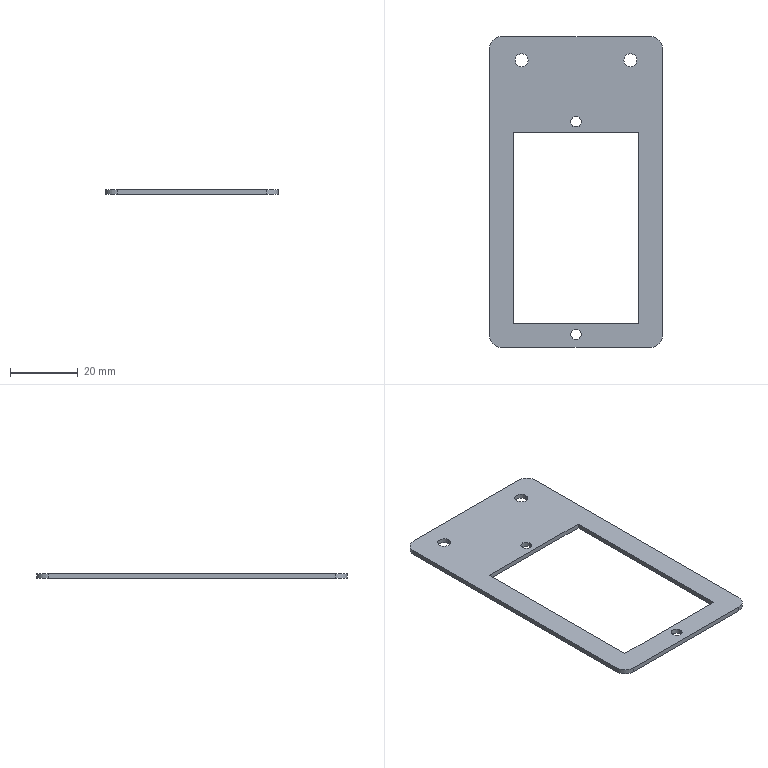Part | SolidWorks | features SplitBody 1 | 1 solid | 22 faces | box 51.1 x 92.05 x 1.4 mm | volume 3571 mm3 | cylinder 12 | plane 10 | commonest cylinder face diameters 3.15 x4 3.85 x4 7 x4
STEP:
#1=CARTESIAN_POINT('',(148.95,235.859,-257.316));
#2=VERTEX_POINT('',#1);
#3=CARTESIAN_POINT('',(152.8,235.859,-257.316));
#4=VERTEX_POINT('',#3);
#5=CARTESIAN_POINT('',(150.875,235.859,-257.316));
#6=DIRECTION('',(0.,0.,1.));
#7=DIRECTION('',(-1.,0.,0.));
#8=AXIS2_PLACEMENT_3D('',#5,#6,#7);
#9=CIRCLE('',#8,1.925);
#10=EDGE_CURVE('',#2,#4,#9,.T.);
#11=ORIENTED_EDGE('',*,*,#10,.F.);
#12=CARTESIAN_POINT('',(148.95,235.859,-255.916));
#13=VERTEX_POINT('',#12);
#14=CARTESIAN_POINT('',(148.95,235.859,-257.316));
#15=DIRECTION('',(0.,0.,1.));
#16=VECTOR('',#15,1000.);
#17=LINE('',#14,#16);
#18=EDGE_CURVE('',#2,#13,#17,.T.);
#19=ORIENTED_EDGE('',*,*,#18,.T.);
#20=CARTESIAN_POINT('',(152.8,235.859,-255.916));
#21=VERTEX_POINT('',#20);
#22=CARTESIAN_POINT('',(150.875,235.859,-255.916));
#23=DIRECTION('',(0.,0.,1.));
#24=DIRECTION('',(-1.,0.,0.));
#25=AXIS2_PLACEMENT_3D('',#22,#23,#24);
#26=CIRCLE('',#25,1.925);
#27=EDGE_CURVE('',#13,#21,#26,.T.);
#28=ORIENTED_EDGE('',*,*,#27,.T.);
#29=CARTESIAN_POINT('',(152.8,235.859,-257.316));
#30=DIRECTION('',(0.,0.,1.));
#31=VECTOR('',#30,1000.);
#32=LINE('',#29,#31);
#33=EDGE_CURVE('',#4,#21,#32,.T.);
#34=ORIENTED_EDGE('',*,*,#33,.F.);
#35=EDGE_LOOP('',(#11,#19,#28,#34));
#36=FACE_OUTER_BOUND('',#35,.T.);
#37=CARTESIAN_POINT('',(150.875,235.859,-257.316));
#38=DIRECTION('',(0.,0.,1.));
#39=DIRECTION('',(1.,0.,0.));
#40=AXIS2_PLACEMENT_3D('',#37,#38,#39);
#41=CYLINDRICAL_SURFACE('',#40,1.925);
#42=ADVANCED_FACE('',(#36),#41,.F.);
#43=CARTESIAN_POINT('',(116.75,235.859,-257.316));
#44=VERTEX_POINT('',#43);
#45=CARTESIAN_POINT('',(120.6,235.859,-257.316));
#46=VERTEX_POINT('',#45);
#47=CARTESIAN_POINT('',(118.675,235.859,-257.316));
#48=DIRECTION('',(0.,0.,1.));
#49=DIRECTION('',(1.,0.,0.));
#50=AXIS2_PLACEMENT_3D('',#47,#48,#49);
#51=CIRCLE('',#50,1.925);
#52=EDGE_CURVE('',#44,#46,#51,.T.);
#53=ORIENTED_EDGE('',*,*,#52,.F.);
#54=CARTESIAN_POINT('',(116.75,235.859,-255.916));
#55=VERTEX_POINT('',#54);
#56=CARTESIAN_POINT('',(116.75,235.859,-257.316));
#57=DIRECTION('',(0.,0.,1.));
#58=VECTOR('',#57,1000.);
#59=LINE('',#56,#58);
#60=EDGE_CURVE('',#44,#55,#59,.T.);
#61=ORIENTED_EDGE('',*,*,#60,.T.);
#62=CARTESIAN_POINT('',(120.6,235.859,-255.916));
#63=VERTEX_POINT('',#62);
#64=CARTESIAN_POINT('',(118.675,235.859,-255.916));
#65=DIRECTION('',(0.,0.,1.));
#66=DIRECTION('',(1.,0.,0.));
#67=AXIS2_PLACEMENT_3D('',#64,#65,#66);
#68=CIRCLE('',#67,1.925);
#69=EDGE_CURVE('',#55,#63,#68,.T.);
#70=ORIENTED_EDGE('',*,*,#69,.T.);
#71=CARTESIAN_POINT('',(120.6,235.859,-257.316));
#72=DIRECTION('',(0.,0.,1.));
#73=VECTOR('',#72,1000.);
#74=LINE('',#71,#73);
#75=EDGE_CURVE('',#46,#63,#74,.T.);
#76=ORIENTED_EDGE('',*,*,#75,.F.);
#77=EDGE_LOOP('',(#53,#61,#70,#76));
#78=FACE_OUTER_BOUND('',#77,.T.);
#79=CARTESIAN_POINT('',(118.675,235.859,-257.316));
#80=DIRECTION('',(0.,0.,1.));
#81=DIRECTION('',(1.,0.,0.));
#82=AXIS2_PLACEMENT_3D('',#79,#80,#81);
#83=CYLINDRICAL_SURFACE('',#82,1.925);
#84=ADVANCED_FACE('',(#78),#83,.F.);
#85=CARTESIAN_POINT('',(133.2,154.659,-257.316));
#86=VERTEX_POINT('',#85);
#87=CARTESIAN_POINT('',(136.35,154.659,-257.316));
#88=VERTEX_POINT('',#87);
#89=CARTESIAN_POINT('',(134.775,154.659,-257.316));
#90=DIRECTION('',(0.,0.,1.));
#91=DIRECTION('',(1.,0.,0.));
#92=AXIS2_PLACEMENT_3D('',#89,#90,#91);
#93=CIRCLE('',#92,1.575);
#94=EDGE_CURVE('',#86,#88,#93,.T.);
#95=ORIENTED_EDGE('',*,*,#94,.F.);
#96=CARTESIAN_POINT('',(133.2,154.659,-255.916));
#97=VERTEX_POINT('',#96);
#98=CARTESIAN_POINT('',(133.2,154.659,-257.316));
#99=DIRECTION('',(0.,0.,1.));
#100=VECTOR('',#99,1000.);
#101=LINE('',#98,#100);
#102=EDGE_CURVE('',#86,#97,#101,.T.);
#103=ORIENTED_EDGE('',*,*,#102,.T.);
#104=CARTESIAN_POINT('',(136.35,154.659,-255.916));
#105=VERTEX_POINT('',#104);
#106=CARTESIAN_POINT('',(134.775,154.659,-255.916));
#107=DIRECTION('',(0.,0.,1.));
#108=DIRECTION('',(1.,0.,0.));
#109=AXIS2_PLACEMENT_3D('',#106,#107,#108);
#110=CIRCLE('',#109,1.575);
#111=EDGE_CURVE('',#97,#105,#110,.T.);
#112=ORIENTED_EDGE('',*,*,#111,.T.);
#113=CARTESIAN_POINT('',(136.35,154.659,-257.316));
#114=DIRECTION('',(0.,0.,1.));
#115=VECTOR('',#114,1000.);
#116=LINE('',#113,#115);
#117=EDGE_CURVE('',#88,#105,#116,.T.);
#118=ORIENTED_EDGE('',*,*,#117,.F.);
#119=EDGE_LOOP('',(#95,#103,#112,#118));
#120=FACE_OUTER_BOUND('',#119,.T.);
#121=CARTESIAN_POINT('',(134.775,154.659,-257.316));
#122=DIRECTION('',(0.,0.,1.));
#123=DIRECTION('',(1.,0.,0.));
#124=AXIS2_PLACEMENT_3D('',#121,#122,#123);
#125=CYLINDRICAL_SURFACE('',#124,1.575);
#126=ADVANCED_FACE('',(#120),#125,.F.);
#127=CARTESIAN_POINT('',(133.2,217.659,-257.316));
#128=VERTEX_POINT('',#127);
#129=CARTESIAN_POINT('',(136.35,217.659,-257.316));
#130=VERTEX_POINT('',#129);
#131=CARTESIAN_POINT('',(134.775,217.659,-257.316));
#132=DIRECTION('',(0.,0.,1.));
#133=DIRECTION('',(1.,0.,0.));
#134=AXIS2_PLACEMENT_3D('',#131,#132,#133);
#135=CIRCLE('',#134,1.575);
#136=EDGE_CURVE('',#128,#130,#135,.T.);
#137=ORIENTED_EDGE('',*,*,#136,.F.);
#138=CARTESIAN_POINT('',(133.2,217.659,-255.916));
#139=VERTEX_POINT('',#138);
#140=CARTESIAN_POINT('',(133.2,217.659,-257.316));
#141=DIRECTION('',(0.,0.,1.));
#142=VECTOR('',#141,1000.);
#143=LINE('',#140,#142);
#144=EDGE_CURVE('',#128,#139,#143,.T.);
#145=ORIENTED_EDGE('',*,*,#144,.T.);
#146=CARTESIAN_POINT('',(136.35,217.659,-255.916));
#147=VERTEX_POINT('',#146);
#148=CARTESIAN_POINT('',(134.775,217.659,-255.916));
#149=DIRECTION('',(0.,0.,1.));
#150=DIRECTION('',(1.,0.,0.));
#151=AXIS2_PLACEMENT_3D('',#148,#149,#150);
#152=CIRCLE('',#151,1.575);
#153=EDGE_CURVE('',#139,#147,#152,.T.);
#154=ORIENTED_EDGE('',*,*,#153,.T.);
#155=CARTESIAN_POINT('',(136.35,217.659,-257.316));
#156=DIRECTION('',(0.,0.,1.));
#157=VECTOR('',#156,1000.);
#158=LINE('',#155,#157);
#159=EDGE_CURVE('',#130,#147,#158,.T.);
#160=ORIENTED_EDGE('',*,*,#159,.F.);
#161=EDGE_LOOP('',(#137,#145,#154,#160));
#162=FACE_OUTER_BOUND('',#161,.T.);
#163=CARTESIAN_POINT('',(134.775,217.659,-257.316));
#164=DIRECTION('',(0.,0.,1.));
#165=DIRECTION('',(1.,0.,0.));
#166=AXIS2_PLACEMENT_3D('',#163,#164,#165);
#167=CYLINDRICAL_SURFACE('',#166,1.575);
#168=ADVANCED_FACE('',(#162),#167,.F.);
#169=CARTESIAN_POINT('',(112.725,150.809,-257.316));
#170=VERTEX_POINT('',#169);
#171=CARTESIAN_POINT('',(156.825,150.809,-257.316));
#172=VERTEX_POINT('',#171);
#173=CARTESIAN_POINT('',(160.325,150.809,-257.316));
#174=DIRECTION('',(1.,0.,0.));
#175=VECTOR('',#174,1000.);
#176=LINE('',#173,#175);
#177=EDGE_CURVE('',#170,#172,#176,.T.);
#178=ORIENTED_EDGE('',*,*,#177,.F.);
#179=CARTESIAN_POINT('',(109.225,154.309,-257.316));
#180=VERTEX_POINT('',#179);
#181=CARTESIAN_POINT('',(112.725,154.309,-257.316));
#182=DIRECTION('',(0.,0.,-1.));
#183=DIRECTION('',(-1.,0.,0.));
#184=AXIS2_PLACEMENT_3D('',#181,#182,#183);
#185=CIRCLE('',#184,3.5);
#186=EDGE_CURVE('',#170,#180,#185,.T.);
#187=ORIENTED_EDGE('',*,*,#186,.T.);
#188=CARTESIAN_POINT('',(109.225,239.359,-257.316));
#189=VERTEX_POINT('',#188);
#190=CARTESIAN_POINT('',(109.225,227.459,-257.316));
#191=DIRECTION('',(0.,1.,0.));
#192=VECTOR('',#191,1000.);
#193=LINE('',#190,#192);
#194=EDGE_CURVE('',#180,#189,#193,.T.);
#195=ORIENTED_EDGE('',*,*,#194,.T.);
#196=CARTESIAN_POINT('',(112.725,242.859,-257.316));
#197=VERTEX_POINT('',#196);
#198=CARTESIAN_POINT('',(112.725,239.359,-257.316));
#199=DIRECTION('',(0.,0.,-1.));
#200=DIRECTION('',(-1.,0.,0.));
#201=AXIS2_PLACEMENT_3D('',#198,#199,#200);
#202=CIRCLE('',#201,3.5);
#203=EDGE_CURVE('',#189,#197,#202,.T.);
#204=ORIENTED_EDGE('',*,*,#203,.T.);
#205=CARTESIAN_POINT('',(156.825,242.859,-257.316));
#206=VERTEX_POINT('',#205);
#207=CARTESIAN_POINT('',(160.325,242.859,-257.316));
#208=DIRECTION('',(1.,0.,0.));
#209=VECTOR('',#208,1000.);
#210=LINE('',#207,#209);
#211=EDGE_CURVE('',#197,#206,#210,.T.);
#212=ORIENTED_EDGE('',*,*,#211,.T.);
#213=CARTESIAN_POINT('',(160.325,239.359,-257.316));
#214=VERTEX_POINT('',#213);
#215=CARTESIAN_POINT('',(156.825,239.359,-257.316));
#216=DIRECTION('',(0.,0.,-1.));
#217=DIRECTION('',(-1.,0.,0.));
#218=AXIS2_PLACEMENT_3D('',#215,#216,#217);
#219=CIRCLE('',#218,3.5);
#220=EDGE_CURVE('',#206,#214,#219,.T.);
#221=ORIENTED_EDGE('',*,*,#220,.T.);
#222=CARTESIAN_POINT('',(160.325,154.309,-257.316));
#223=VERTEX_POINT('',#222);
#224=CARTESIAN_POINT('',(160.325,227.459,-257.316));
#225=DIRECTION('',(0.,-1.,0.));
#226=VECTOR('',#225,1000.);
#227=LINE('',#224,#226);
#228=EDGE_CURVE('',#214,#223,#227,.T.);
#229=ORIENTED_EDGE('',*,*,#228,.T.);
#230=CARTESIAN_POINT('',(156.825,154.309,-257.316));
#231=DIRECTION('',(0.,0.,-1.));
#232=DIRECTION('',(-1.,0.,0.));
#233=AXIS2_PLACEMENT_3D('',#230,#231,#232);
#234=CIRCLE('',#233,3.5);
#235=EDGE_CURVE('',#223,#172,#234,.T.);
#236=ORIENTED_EDGE('',*,*,#235,.T.);
#237=EDGE_LOOP('',(#178,#187,#195,#204,#212,#221,#229,#236));
#238=FACE_OUTER_BOUND('',#237,.T.);
#239=CARTESIAN_POINT('',(150.875,235.859,-257.316));
#240=DIRECTION('',(0.,0.,1.));
#241=DIRECTION('',(-1.,0.,0.));
#242=AXIS2_PLACEMENT_3D('',#239,#240,#241);
#243=CIRCLE('',#242,1.925);
#244=EDGE_CURVE('',#4,#2,#243,.T.);
#245=ORIENTED_EDGE('',*,*,#244,.T.);
#246=ORIENTED_EDGE('',*,*,#10,.T.);
#247=EDGE_LOOP('',(#245,#246));
#248=FACE_BOUND('',#247,.T.);
#249=CARTESIAN_POINT('',(118.675,235.859,-257.316));
#250=DIRECTION('',(0.,0.,1.));
#251=DIRECTION('',(1.,0.,0.));
#252=AXIS2_PLACEMENT_3D('',#249,#250,#251);
#253=CIRCLE('',#252,1.925);
#254=EDGE_CURVE('',#46,#44,#253,.T.);
#255=ORIENTED_EDGE('',*,*,#254,.T.);
#256=ORIENTED_EDGE('',*,*,#52,.T.);
#257=EDGE_LOOP('',(#255,#256));
#258=FACE_BOUND('',#257,.T.);
#259=CARTESIAN_POINT('',(134.775,154.659,-257.316));
#260=DIRECTION('',(0.,0.,1.));
#261=DIRECTION('',(1.,0.,0.));
#262=AXIS2_PLACEMENT_3D('',#259,#260,#261);
#263=CIRCLE('',#262,1.575);
#264=EDGE_CURVE('',#88,#86,#263,.T.);
#265=ORIENTED_EDGE('',*,*,#264,.T.);
#266=ORIENTED_EDGE('',*,*,#94,.T.);
#267=EDGE_LOOP('',(#265,#266));
#268=FACE_BOUND('',#267,.T.);
#269=CARTESIAN_POINT('',(134.775,217.659,-257.316));
#270=DIRECTION('',(0.,0.,1.));
#271=DIRECTION('',(1.,0.,0.));
#272=AXIS2_PLACEMENT_3D('',#269,#270,#271);
#273=CIRCLE('',#272,1.575);
#274=EDGE_CURVE('',#130,#128,#273,.T.);
#275=ORIENTED_EDGE('',*,*,#274,.T.);
#276=ORIENTED_EDGE('',*,*,#136,.T.);
#277=EDGE_LOOP('',(#275,#276));
#278=FACE_BOUND('',#277,.T.);
#279=CARTESIAN_POINT('',(153.325,214.509,-257.316));
#280=VERTEX_POINT('',#279);
#281=CARTESIAN_POINT('',(153.325,157.809,-257.316));
#282=VERTEX_POINT('',#281);
#283=CARTESIAN_POINT('',(153.325,220.459,-257.316));
#284=DIRECTION('',(0.,-1.,0.));
#285=VECTOR('',#284,1000.);
#286=LINE('',#283,#285);
#287=EDGE_CURVE('',#280,#282,#286,.T.);
#288=ORIENTED_EDGE('',*,*,#287,.F.);
#289=CARTESIAN_POINT('',(116.225,214.509,-257.316));
#290=VERTEX_POINT('',#289);
#291=CARTESIAN_POINT('',(153.325,214.509,-257.316));
#292=DIRECTION('',(-1.,0.,0.));
#293=VECTOR('',#292,1000.);
#294=LINE('',#291,#293);
#295=EDGE_CURVE('',#280,#290,#294,.T.);
#296=ORIENTED_EDGE('',*,*,#295,.T.);
#297=CARTESIAN_POINT('',(116.225,157.809,-257.316));
#298=VERTEX_POINT('',#297);
#299=CARTESIAN_POINT('',(116.225,220.459,-257.316));
#300=DIRECTION('',(0.,1.,0.));
#301=VECTOR('',#300,1000.);
#302=LINE('',#299,#301);
#303=EDGE_CURVE('',#298,#290,#302,.T.);
#304=ORIENTED_EDGE('',*,*,#303,.F.);
#305=CARTESIAN_POINT('',(153.325,157.809,-257.316));
#306=DIRECTION('',(1.,0.,0.));
#307=VECTOR('',#306,1000.);
#308=LINE('',#305,#307);
#309=EDGE_CURVE('',#298,#282,#308,.T.);
#310=ORIENTED_EDGE('',*,*,#309,.T.);
#311=EDGE_LOOP('',(#288,#296,#304,#310));
#312=FACE_BOUND('',#311,.T.);
#313=CARTESIAN_POINT('',(160.325,144.859,-257.316));
#314=DIRECTION('',(0.,0.,-1.));
#315=DIRECTION('',(-1.,0.,0.));
#316=AXIS2_PLACEMENT_3D('',#313,#314,#315);
#317=PLANE('',#316);
#318=ADVANCED_FACE('',(#238,#248,#258,#268,#278,#312),#317,.T.);
#319=CARTESIAN_POINT('',(150.875,235.859,-255.916));
#320=DIRECTION('',(0.,0.,1.));
#321=DIRECTION('',(-1.,0.,0.));
#322=AXIS2_PLACEMENT_3D('',#319,#320,#321);
#323=CIRCLE('',#322,1.925);
#324=EDGE_CURVE('',#21,#13,#323,.T.);
#325=ORIENTED_EDGE('',*,*,#324,.F.);
#326=ORIENTED_EDGE('',*,*,#27,.F.);
#327=EDGE_LOOP('',(#325,#326));
#328=FACE_BOUND('',#327,.T.);
#329=CARTESIAN_POINT('',(118.675,235.859,-255.916));
#330=DIRECTION('',(0.,0.,1.));
#331=DIRECTION('',(1.,0.,0.));
#332=AXIS2_PLACEMENT_3D('',#329,#330,#331);
#333=CIRCLE('',#332,1.925);
#334=EDGE_CURVE('',#63,#55,#333,.T.);
#335=ORIENTED_EDGE('',*,*,#334,.F.);
#336=ORIENTED_EDGE('',*,*,#69,.F.);
#337=EDGE_LOOP('',(#335,#336));
#338=FACE_BOUND('',#337,.T.);
#339=CARTESIAN_POINT('',(134.775,154.659,-255.916));
#340=DIRECTION('',(0.,0.,1.));
#341=DIRECTION('',(1.,0.,0.));
#342=AXIS2_PLACEMENT_3D('',#339,#340,#341);
#343=CIRCLE('',#342,1.575);
#344=EDGE_CURVE('',#105,#97,#343,.T.);
#345=ORIENTED_EDGE('',*,*,#344,.F.);
#346=ORIENTED_EDGE('',*,*,#111,.F.);
#347=EDGE_LOOP('',(#345,#346));
#348=FACE_BOUND('',#347,.T.);
#349=CARTESIAN_POINT('',(134.775,217.659,-255.916));
#350=DIRECTION('',(0.,0.,1.));
#351=DIRECTION('',(1.,0.,0.));
#352=AXIS2_PLACEMENT_3D('',#349,#350,#351);
#353=CIRCLE('',#352,1.575);
#354=EDGE_CURVE('',#147,#139,#353,.T.);
#355=ORIENTED_EDGE('',*,*,#354,.F.);
#356=ORIENTED_EDGE('',*,*,#153,.F.);
#357=EDGE_LOOP('',(#355,#356));
#358=FACE_BOUND('',#357,.T.);
#359=CARTESIAN_POINT('',(116.225,214.509,-255.916));
#360=VERTEX_POINT('',#359);
#361=CARTESIAN_POINT('',(153.325,214.509,-255.916));
#362=VERTEX_POINT('',#361);
#363=CARTESIAN_POINT('',(153.325,214.509,-255.916));
#364=DIRECTION('',(1.,0.,0.));
#365=VECTOR('',#364,1000.);
#366=LINE('',#363,#365);
#367=EDGE_CURVE('',#360,#362,#366,.T.);
#368=ORIENTED_EDGE('',*,*,#367,.T.);
#369=CARTESIAN_POINT('',(153.325,157.809,-255.916));
#370=VERTEX_POINT('',#369);
#371=CARTESIAN_POINT('',(153.325,220.459,-255.916));
#372=DIRECTION('',(0.,-1.,0.));
#373=VECTOR('',#372,1000.);
#374=LINE('',#371,#373);
#375=EDGE_CURVE('',#362,#370,#374,.T.);
#376=ORIENTED_EDGE('',*,*,#375,.T.);
#377=CARTESIAN_POINT('',(116.225,157.809,-255.916));
#378=VERTEX_POINT('',#377);
#379=CARTESIAN_POINT('',(153.325,157.809,-255.916));
#380=DIRECTION('',(-1.,0.,0.));
#381=VECTOR('',#380,1000.);
#382=LINE('',#379,#381);
#383=EDGE_CURVE('',#370,#378,#382,.T.);
#384=ORIENTED_EDGE('',*,*,#383,.T.);
#385=CARTESIAN_POINT('',(116.225,220.459,-255.916));
#386=DIRECTION('',(0.,1.,0.));
#387=VECTOR('',#386,1000.);
#388=LINE('',#385,#387);
#389=EDGE_CURVE('',#378,#360,#388,.T.);
#390=ORIENTED_EDGE('',*,*,#389,.T.);
#391=EDGE_LOOP('',(#368,#376,#384,#390));
#392=FACE_BOUND('',#391,.T.);
#393=CARTESIAN_POINT('',(109.225,154.309,-255.916));
#394=VERTEX_POINT('',#393);
#395=CARTESIAN_POINT('',(109.225,239.359,-255.916));
#396=VERTEX_POINT('',#395);
#397=CARTESIAN_POINT('',(109.225,227.459,-255.916));
#398=DIRECTION('',(0.,1.,0.));
#399=VECTOR('',#398,1000.);
#400=LINE('',#397,#399);
#401=EDGE_CURVE('',#394,#396,#400,.T.);
#402=ORIENTED_EDGE('',*,*,#401,.F.);
#403=CARTESIAN_POINT('',(112.725,150.809,-255.916));
#404=VERTEX_POINT('',#403);
#405=CARTESIAN_POINT('',(112.725,154.309,-255.916));
#406=DIRECTION('',(0.,0.,1.));
#407=DIRECTION('',(-1.,0.,0.));
#408=AXIS2_PLACEMENT_3D('',#405,#406,#407);
#409=CIRCLE('',#408,3.5);
#410=EDGE_CURVE('',#394,#404,#409,.T.);
#411=ORIENTED_EDGE('',*,*,#410,.T.);
#412=CARTESIAN_POINT('',(156.825,150.809,-255.916));
#413=VERTEX_POINT('',#412);
#414=CARTESIAN_POINT('',(160.325,150.809,-255.916));
#415=DIRECTION('',(1.,0.,0.));
#416=VECTOR('',#415,1000.);
#417=LINE('',#414,#416);
#418=EDGE_CURVE('',#404,#413,#417,.T.);
#419=ORIENTED_EDGE('',*,*,#418,.T.);
#420=CARTESIAN_POINT('',(160.325,154.309,-255.916));
#421=VERTEX_POINT('',#420);
#422=CARTESIAN_POINT('',(156.825,154.309,-255.916));
#423=DIRECTION('',(0.,0.,1.));
#424=DIRECTION('',(-1.,0.,0.));
#425=AXIS2_PLACEMENT_3D('',#422,#423,#424);
#426=CIRCLE('',#425,3.5);
#427=EDGE_CURVE('',#413,#421,#426,.T.);
#428=ORIENTED_EDGE('',*,*,#427,.T.);
#429=CARTESIAN_POINT('',(160.325,239.359,-255.916));
#430=VERTEX_POINT('',#429);
#431=CARTESIAN_POINT('',(160.325,227.459,-255.916));
#432=DIRECTION('',(0.,-1.,0.));
#433=VECTOR('',#432,1000.);
#434=LINE('',#431,#433);
#435=EDGE_CURVE('',#430,#421,#434,.T.);
#436=ORIENTED_EDGE('',*,*,#435,.F.);
#437=CARTESIAN_POINT('',(156.825,242.859,-255.916));
#438=VERTEX_POINT('',#437);
#439=CARTESIAN_POINT('',(156.825,239.359,-255.916));
#440=DIRECTION('',(0.,0.,1.));
#441=DIRECTION('',(-1.,0.,0.));
#442=AXIS2_PLACEMENT_3D('',#439,#440,#441);
#443=CIRCLE('',#442,3.5);
#444=EDGE_CURVE('',#430,#438,#443,.T.);
#445=ORIENTED_EDGE('',*,*,#444,.T.);
#446=CARTESIAN_POINT('',(112.725,242.859,-255.916));
#447=VERTEX_POINT('',#446);
#448=CARTESIAN_POINT('',(160.325,242.859,-255.916));
#449=DIRECTION('',(-1.,0.,0.));
#450=VECTOR('',#449,1000.);
#451=LINE('',#448,#450);
#452=EDGE_CURVE('',#438,#447,#451,.T.);
#453=ORIENTED_EDGE('',*,*,#452,.T.);
#454=CARTESIAN_POINT('',(112.725,239.359,-255.916));
#455=DIRECTION('',(0.,0.,1.));
#456=DIRECTION('',(-1.,0.,0.));
#457=AXIS2_PLACEMENT_3D('',#454,#455,#456);
#458=CIRCLE('',#457,3.5);
#459=EDGE_CURVE('',#447,#396,#458,.T.);
#460=ORIENTED_EDGE('',*,*,#459,.T.);
#461=EDGE_LOOP('',(#402,#411,#419,#428,#436,#445,#453,#460));
#462=FACE_OUTER_BOUND('',#461,.T.);
#463=CARTESIAN_POINT('',(160.325,144.859,-255.916));
#464=DIRECTION('',(0.,0.,-1.));
#465=DIRECTION('',(-1.,0.,0.));
#466=AXIS2_PLACEMENT_3D('',#463,#464,#465);
#467=PLANE('',#466);
#468=ADVANCED_FACE('',(#328,#338,#348,#358,#392,#462),#467,.F.);
#469=ORIENTED_EDGE('',*,*,#435,.T.);
#470=CARTESIAN_POINT('',(160.325,154.309,-257.316));
#471=DIRECTION('',(0.,0.,-1.));
#472=VECTOR('',#471,1000.);
#473=LINE('',#470,#472);
#474=EDGE_CURVE('',#421,#223,#473,.T.);
#475=ORIENTED_EDGE('',*,*,#474,.T.);
#476=ORIENTED_EDGE('',*,*,#228,.F.);
#477=CARTESIAN_POINT('',(160.325,239.359,-255.916));
#478=DIRECTION('',(0.,0.,1.));
#479=VECTOR('',#478,1000.);
#480=LINE('',#477,#479);
#481=EDGE_CURVE('',#214,#430,#480,.T.);
#482=ORIENTED_EDGE('',*,*,#481,.T.);
#483=EDGE_LOOP('',(#469,#475,#476,#482));
#484=FACE_OUTER_BOUND('',#483,.T.);
#485=CARTESIAN_POINT('',(160.325,227.459,-257.316));
#486=DIRECTION('',(-1.,0.,0.));
#487=DIRECTION('',(0.,0.,1.));
#488=AXIS2_PLACEMENT_3D('',#485,#486,#487);
#489=PLANE('',#488);
#490=ADVANCED_FACE('',(#484),#489,.F.);
#491=ORIENTED_EDGE('',*,*,#194,.F.);
#492=CARTESIAN_POINT('',(109.225,154.309,-257.316));
#493=DIRECTION('',(0.,0.,1.));
#494=VECTOR('',#493,1000.);
#495=LINE('',#492,#494);
#496=EDGE_CURVE('',#180,#394,#495,.T.);
#497=ORIENTED_EDGE('',*,*,#496,.T.);
#498=ORIENTED_EDGE('',*,*,#401,.T.);
#499=CARTESIAN_POINT('',(109.225,239.359,-257.316));
#500=DIRECTION('',(0.,0.,-1.));
#501=VECTOR('',#500,1000.);
#502=LINE('',#499,#501);
#503=EDGE_CURVE('',#396,#189,#502,.T.);
#504=ORIENTED_EDGE('',*,*,#503,.T.);
#505=EDGE_LOOP('',(#491,#497,#498,#504));
#506=FACE_OUTER_BOUND('',#505,.T.);
#507=CARTESIAN_POINT('',(109.225,227.459,-257.316));
#508=DIRECTION('',(1.,0.,0.));
#509=DIRECTION('',(0.,0.,-1.));
#510=AXIS2_PLACEMENT_3D('',#507,#508,#509);
#511=PLANE('',#510);
#512=ADVANCED_FACE('',(#506),#511,.F.);
#513=CARTESIAN_POINT('',(153.325,214.509,-218.342));
#514=DIRECTION('',(0.,0.,-1.));
#515=VECTOR('',#514,1000.);
#516=LINE('',#513,#515);
#517=EDGE_CURVE('',#362,#280,#516,.T.);
#518=ORIENTED_EDGE('',*,*,#517,.T.);
#519=ORIENTED_EDGE('',*,*,#287,.T.);
#520=CARTESIAN_POINT('',(153.325,157.809,-218.342));
#521=DIRECTION('',(0.,0.,-1.));
#522=VECTOR('',#521,1000.);
#523=LINE('',#520,#522);
#524=EDGE_CURVE('',#370,#282,#523,.T.);
#525=ORIENTED_EDGE('',*,*,#524,.F.);
#526=ORIENTED_EDGE('',*,*,#375,.F.);
#527=EDGE_LOOP('',(#518,#519,#525,#526));
#528=FACE_OUTER_BOUND('',#527,.T.);
#529=CARTESIAN_POINT('',(153.325,220.459,-257.316));
#530=DIRECTION('',(-1.,0.,0.));
#531=DIRECTION('',(0.,1.,0.));
#532=AXIS2_PLACEMENT_3D('',#529,#530,#531);
#533=PLANE('',#532);
#534=ADVANCED_FACE('',(#528),#533,.T.);
#535=CARTESIAN_POINT('',(116.225,214.509,-218.342));
#536=DIRECTION('',(0.,0.,-1.));
#537=VECTOR('',#536,1000.);
#538=LINE('',#535,#537);
#539=EDGE_CURVE('',#360,#290,#538,.T.);
#540=ORIENTED_EDGE('',*,*,#539,.F.);
#541=ORIENTED_EDGE('',*,*,#389,.F.);
#542=CARTESIAN_POINT('',(116.225,157.809,-218.342));
#543=DIRECTION('',(0.,0.,-1.));
#544=VECTOR('',#543,1000.);
#545=LINE('',#542,#544);
#546=EDGE_CURVE('',#378,#298,#545,.T.);
#547=ORIENTED_EDGE('',*,*,#546,.T.);
#548=ORIENTED_EDGE('',*,*,#303,.T.);
#549=EDGE_LOOP('',(#540,#541,#547,#548));
#550=FACE_OUTER_BOUND('',#549,.T.);
#551=CARTESIAN_POINT('',(116.225,220.459,-257.316));
#552=DIRECTION('',(1.,0.,0.));
#553=DIRECTION('',(0.,0.,-1.));
#554=AXIS2_PLACEMENT_3D('',#551,#552,#553);
#555=PLANE('',#554);
#556=ADVANCED_FACE('',(#550),#555,.T.);
#557=ORIENTED_EDGE('',*,*,#383,.F.);
#558=ORIENTED_EDGE('',*,*,#524,.T.);
#559=ORIENTED_EDGE('',*,*,#309,.F.);
#560=ORIENTED_EDGE('',*,*,#546,.F.);
#561=EDGE_LOOP('',(#557,#558,#559,#560));
#562=FACE_OUTER_BOUND('',#561,.T.);
#563=CARTESIAN_POINT('',(153.325,157.809,-218.342));
#564=DIRECTION('',(0.,1.,0.));
#565=DIRECTION('',(0.,0.,-1.));
#566=AXIS2_PLACEMENT_3D('',#563,#564,#565);
#567=PLANE('',#566);
#568=ADVANCED_FACE('',(#562),#567,.T.);
#569=ORIENTED_EDGE('',*,*,#367,.F.);
#570=ORIENTED_EDGE('',*,*,#539,.T.);
#571=ORIENTED_EDGE('',*,*,#295,.F.);
#572=ORIENTED_EDGE('',*,*,#517,.F.);
#573=EDGE_LOOP('',(#569,#570,#571,#572));
#574=FACE_OUTER_BOUND('',#573,.T.);
#575=CARTESIAN_POINT('',(153.325,214.509,-218.342));
#576=DIRECTION('',(0.,-1.,0.));
#577=DIRECTION('',(-1.,0.,0.));
#578=AXIS2_PLACEMENT_3D('',#575,#576,#577);
#579=PLANE('',#578);
#580=ADVANCED_FACE('',(#574),#579,.T.);
#581=ORIENTED_EDGE('',*,*,#211,.F.);
#582=CARTESIAN_POINT('',(112.725,242.859,-255.916));
#583=DIRECTION('',(0.,0.,1.));
#584=VECTOR('',#583,1000.);
#585=LINE('',#582,#584);
#586=EDGE_CURVE('',#197,#447,#585,.T.);
#587=ORIENTED_EDGE('',*,*,#586,.T.);
#588=ORIENTED_EDGE('',*,*,#452,.F.);
#589=CARTESIAN_POINT('',(156.825,242.859,-257.316));
#590=DIRECTION('',(0.,0.,-1.));
#591=VECTOR('',#590,1000.);
#592=LINE('',#589,#591);
#593=EDGE_CURVE('',#438,#206,#592,.T.);
#594=ORIENTED_EDGE('',*,*,#593,.T.);
#595=EDGE_LOOP('',(#581,#587,#588,#594));
#596=FACE_OUTER_BOUND('',#595,.T.);
#597=CARTESIAN_POINT('',(160.325,242.859,-202.545));
#598=DIRECTION('',(0.,1.,0.));
#599=DIRECTION('',(0.,0.,-1.));
#600=AXIS2_PLACEMENT_3D('',#597,#598,#599);
#601=PLANE('',#600);
#602=ADVANCED_FACE('',(#596),#601,.T.);
#603=ORIENTED_EDGE('',*,*,#459,.F.);
#604=ORIENTED_EDGE('',*,*,#586,.F.);
#605=ORIENTED_EDGE('',*,*,#203,.F.);
#606=ORIENTED_EDGE('',*,*,#503,.F.);
#607=EDGE_LOOP('',(#603,#604,#605,#606));
#608=FACE_OUTER_BOUND('',#607,.T.);
#609=CARTESIAN_POINT('',(112.725,239.359,-257.316));
#610=DIRECTION('',(0.,0.,1.));
#611=DIRECTION('',(1.,0.,0.));
#612=AXIS2_PLACEMENT_3D('',#609,#610,#611);
#613=CYLINDRICAL_SURFACE('',#612,3.5);
#614=ADVANCED_FACE('',(#608),#613,.T.);
#615=ORIENTED_EDGE('',*,*,#444,.F.);
#616=ORIENTED_EDGE('',*,*,#481,.F.);
#617=ORIENTED_EDGE('',*,*,#220,.F.);
#618=ORIENTED_EDGE('',*,*,#593,.F.);
#619=EDGE_LOOP('',(#615,#616,#617,#618));
#620=FACE_OUTER_BOUND('',#619,.T.);
#621=CARTESIAN_POINT('',(156.825,239.359,-202.545));
#622=DIRECTION('',(0.,0.,1.));
#623=DIRECTION('',(1.,0.,0.));
#624=AXIS2_PLACEMENT_3D('',#621,#622,#623);
#625=CYLINDRICAL_SURFACE('',#624,3.5);
#626=ADVANCED_FACE('',(#620),#625,.T.);
#627=ORIENTED_EDGE('',*,*,#144,.F.);
#628=ORIENTED_EDGE('',*,*,#274,.F.);
#629=ORIENTED_EDGE('',*,*,#159,.T.);
#630=ORIENTED_EDGE('',*,*,#354,.T.);
#631=EDGE_LOOP('',(#627,#628,#629,#630));
#632=FACE_OUTER_BOUND('',#631,.T.);
#633=CARTESIAN_POINT('',(134.775,217.659,-257.316));
#634=DIRECTION('',(0.,0.,1.));
#635=DIRECTION('',(1.,0.,0.));
#636=AXIS2_PLACEMENT_3D('',#633,#634,#635);
#637=CYLINDRICAL_SURFACE('',#636,1.575);
#638=ADVANCED_FACE('',(#632),#637,.F.);
#639=ORIENTED_EDGE('',*,*,#102,.F.);
#640=ORIENTED_EDGE('',*,*,#264,.F.);
#641=ORIENTED_EDGE('',*,*,#117,.T.);
#642=ORIENTED_EDGE('',*,*,#344,.T.);
#643=EDGE_LOOP('',(#639,#640,#641,#642));
#644=FACE_OUTER_BOUND('',#643,.T.);
#645=CARTESIAN_POINT('',(134.775,154.659,-257.316));
#646=DIRECTION('',(0.,0.,1.));
#647=DIRECTION('',(1.,0.,0.));
#648=AXIS2_PLACEMENT_3D('',#645,#646,#647);
#649=CYLINDRICAL_SURFACE('',#648,1.575);
#650=ADVANCED_FACE('',(#644),#649,.F.);
#651=ORIENTED_EDGE('',*,*,#60,.F.);
#652=ORIENTED_EDGE('',*,*,#254,.F.);
#653=ORIENTED_EDGE('',*,*,#75,.T.);
#654=ORIENTED_EDGE('',*,*,#334,.T.);
#655=EDGE_LOOP('',(#651,#652,#653,#654));
#656=FACE_OUTER_BOUND('',#655,.T.);
#657=CARTESIAN_POINT('',(118.675,235.859,-257.316));
#658=DIRECTION('',(0.,0.,1.));
#659=DIRECTION('',(1.,0.,0.));
#660=AXIS2_PLACEMENT_3D('',#657,#658,#659);
#661=CYLINDRICAL_SURFACE('',#660,1.925);
#662=ADVANCED_FACE('',(#656),#661,.F.);
#663=ORIENTED_EDGE('',*,*,#18,.F.);
#664=ORIENTED_EDGE('',*,*,#244,.F.);
#665=ORIENTED_EDGE('',*,*,#33,.T.);
#666=ORIENTED_EDGE('',*,*,#324,.T.);
#667=EDGE_LOOP('',(#663,#664,#665,#666));
#668=FACE_OUTER_BOUND('',#667,.T.);
#669=CARTESIAN_POINT('',(150.875,235.859,-257.316));
#670=DIRECTION('',(0.,0.,1.));
#671=DIRECTION('',(1.,0.,0.));
#672=AXIS2_PLACEMENT_3D('',#669,#670,#671);
#673=CYLINDRICAL_SURFACE('',#672,1.925);
#674=ADVANCED_FACE('',(#668),#673,.F.);
#675=ORIENTED_EDGE('',*,*,#418,.F.);
#676=CARTESIAN_POINT('',(112.725,150.809,-250.316));
#677=DIRECTION('',(0.,0.,-1.));
#678=VECTOR('',#677,1000.);
#679=LINE('',#676,#678);
#680=EDGE_CURVE('',#404,#170,#679,.T.);
#681=ORIENTED_EDGE('',*,*,#680,.T.);
#682=ORIENTED_EDGE('',*,*,#177,.T.);
#683=CARTESIAN_POINT('',(156.825,150.809,-250.316));
#684=DIRECTION('',(0.,0.,1.));
#685=VECTOR('',#684,1000.);
#686=LINE('',#683,#685);
#687=EDGE_CURVE('',#172,#413,#686,.T.);
#688=ORIENTED_EDGE('',*,*,#687,.T.);
#689=EDGE_LOOP('',(#675,#681,#682,#688));
#690=FACE_OUTER_BOUND('',#689,.T.);
#691=CARTESIAN_POINT('',(160.325,150.809,-250.316));
#692=DIRECTION('',(0.,1.,0.));
#693=DIRECTION('',(1.,0.,0.));
#694=AXIS2_PLACEMENT_3D('',#691,#692,#693);
#695=PLANE('',#694);
#696=ADVANCED_FACE('',(#690),#695,.F.);
#697=ORIENTED_EDGE('',*,*,#186,.F.);
#698=ORIENTED_EDGE('',*,*,#680,.F.);
#699=ORIENTED_EDGE('',*,*,#410,.F.);
#700=ORIENTED_EDGE('',*,*,#496,.F.);
#701=EDGE_LOOP('',(#697,#698,#699,#700));
#702=FACE_OUTER_BOUND('',#701,.T.);
#703=CARTESIAN_POINT('',(112.725,154.309,-257.316));
#704=DIRECTION('',(0.,0.,1.));
#705=DIRECTION('',(1.,0.,0.));
#706=AXIS2_PLACEMENT_3D('',#703,#704,#705);
#707=CYLINDRICAL_SURFACE('',#706,3.5);
#708=ADVANCED_FACE('',(#702),#707,.T.);
#709=ORIENTED_EDGE('',*,*,#427,.F.);
#710=ORIENTED_EDGE('',*,*,#687,.F.);
#711=ORIENTED_EDGE('',*,*,#235,.F.);
#712=ORIENTED_EDGE('',*,*,#474,.F.);
#713=EDGE_LOOP('',(#709,#710,#711,#712));
#714=FACE_OUTER_BOUND('',#713,.T.);
#715=CARTESIAN_POINT('',(156.825,154.309,-257.316));
#716=DIRECTION('',(0.,0.,-1.));
#717=DIRECTION('',(-1.,0.,0.));
#718=AXIS2_PLACEMENT_3D('',#715,#716,#717);
#719=CYLINDRICAL_SURFACE('',#718,3.5);
#720=ADVANCED_FACE('',(#714),#719,.T.);
#721=CLOSED_SHELL('',(#42,#84,#126,#168,#318,#468,#490,#512,#534,#556,#568,#580,#602,#614,#626,#638,#650,#662,#674,#696,#708,#720));
#722=MANIFOLD_SOLID_BREP('',#721);
#723=CARTESIAN_POINT('',(0.,0.,0.));
#724=DIRECTION('',(0.,0.,1.));
#725=DIRECTION('',(1.,0.,0.));
#726=AXIS2_PLACEMENT_3D('',#723,#724,#725);
#727=(LENGTH_UNIT()NAMED_UNIT(*)SI_UNIT(.MILLI.,.METRE.));
#728=UNCERTAINTY_MEASURE_WITH_UNIT(LENGTH_MEASURE(0.00001),#727,'','');
#729=(NAMED_UNIT(*)PLANE_ANGLE_UNIT()SI_UNIT($,.RADIAN.));
#730=(NAMED_UNIT(*)SI_UNIT($,.STERADIAN.)SOLID_ANGLE_UNIT());
#731=(GEOMETRIC_REPRESENTATION_CONTEXT(3)GLOBAL_UNCERTAINTY_ASSIGNED_CONTEXT((#728))GLOBAL_UNIT_ASSIGNED_CONTEXT((#727,#729,#730))REPRESENTATION_CONTEXT('',''));
#732=ADVANCED_BREP_SHAPE_REPRESENTATION('',(#722,#726),#731);